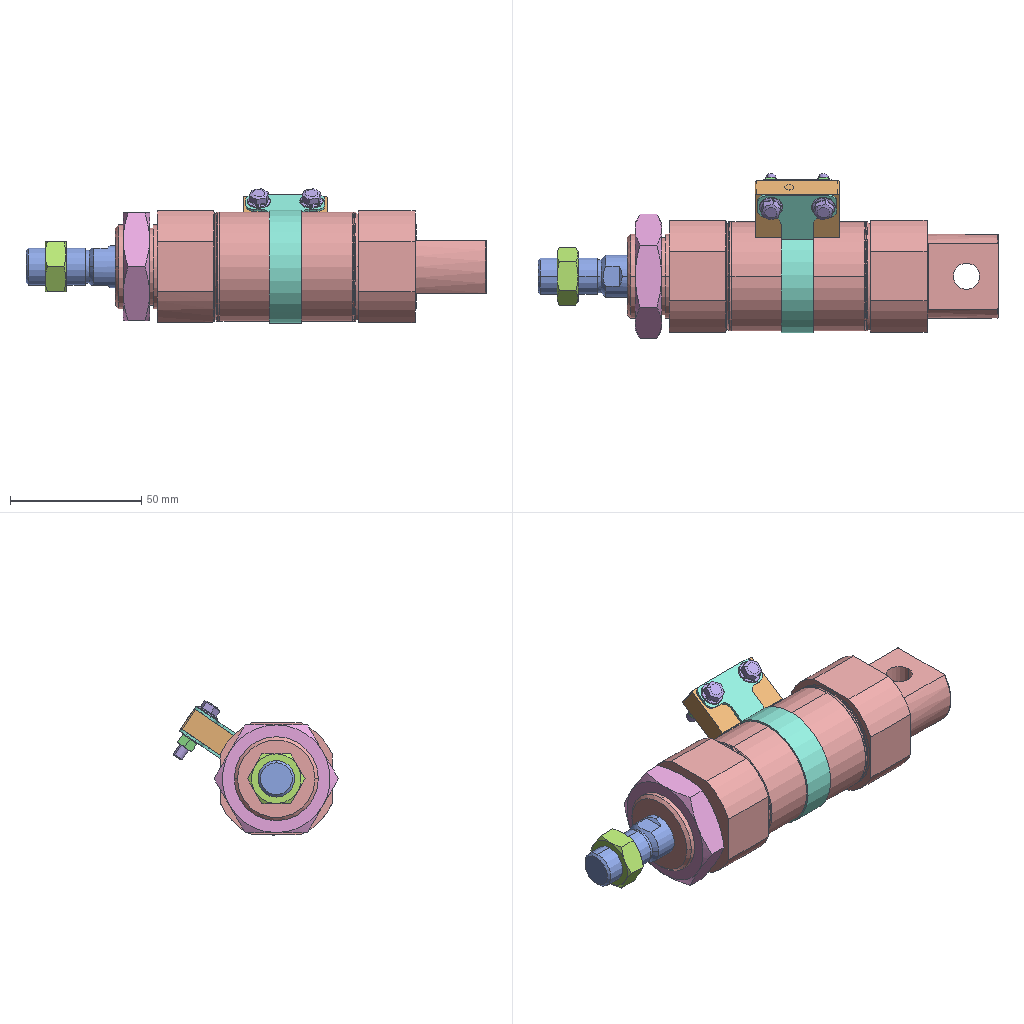Assembly | SolidWorks | 9 different items | 11 placed | box 175 x 63 x 51 mm
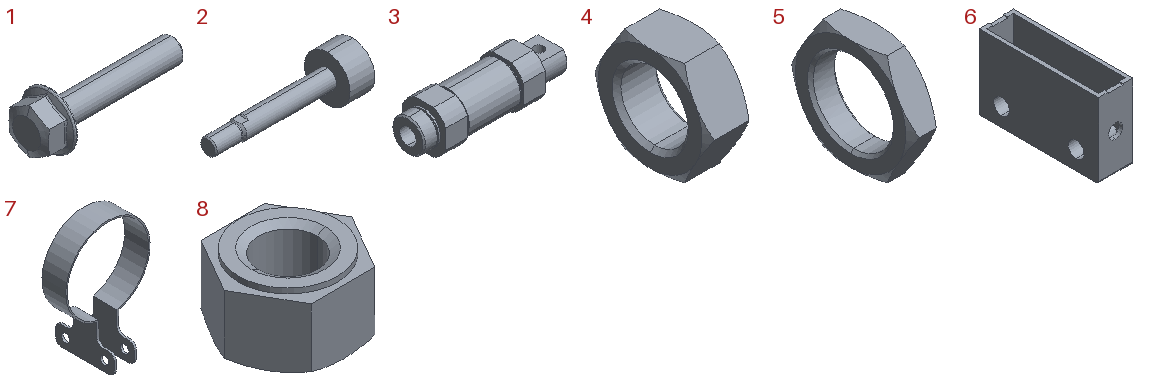Parts list (item | name | quantity | size | volume | features):
1 | - | x2 | 24.05 x 9 x 9 mm | 413.187 mm3 | features BaseBody 1, Scale 1
2 | - | x1 | 125 x 39.5 x 39.5 mm | 45935 mm3 | features BaseBody 1
3 | - | x1 | 141 x 42.5 x 42.5 mm | 117121 mm3 | features BaseBody 1
4 | - | x1 | 8 x 21.939 x 19 mm | 1497 mm3 | features BaseBody 1
5 | - | x1 | 10 x 47.343 x 41 mm | 7305 mm3 | features BaseBody 1
6 | - | x1 | 9.2 x 32 x 20.1 mm | 1950 mm3 | features ICE 8, Fillet 2, Extrusion 1
7 | - | x1 | 43 x 30 x 62.202 mm | 1832 mm3 | features Extrusion 1, ICE 1, MirrorPattern 1
8 | - | x2 | 7.506 x 6.5 x 4.05 mm | 105.396 mm3 | features BaseBody 1, Scale 1
9 | Part5 | x1 | - | - | -
Mates (type | each side: item.copy, entity, surface, feature):
Concentric | 3.1 face cylinder Imported1 | 7.1 face cylinder Boss-Extrude1
Coincident | 7.1 face plane Boss-Extrude1 | 6.1 face plane Boss-Extrude1
Coincident | 3.1 face cylinder Imported1 | 6.1 edge
DistanceDim | 7.1 face plane Mirror1 | 6.1 face plane Boss-Extrude1
Concentric | 6.1 face cylinder Cut-Extrude1 | 1.1 face cylinder Imported1
Coincident | 7.1 face plane Mirror1 | 1.1 face plane Imported1
Concentric | 1.1 face cylinder Imported1 | 8.1 face cylinder Imported1
Coincident | 7.1 face plane Boss-Extrude2 | 8.1 face plane Imported1
Concentric | 1.2 face cylinder Imported1 | 8.2 face cylinder Imported1
Concentric | 6.1 face cylinder Cut-Extrude1 | 1.2 face cylinder Imported1
Coincident | 7.1 face plane Mirror1 | 1.2 face plane Imported1
Coincident | 7.1 face plane Boss-Extrude2 | 8.2 face plane Imported1